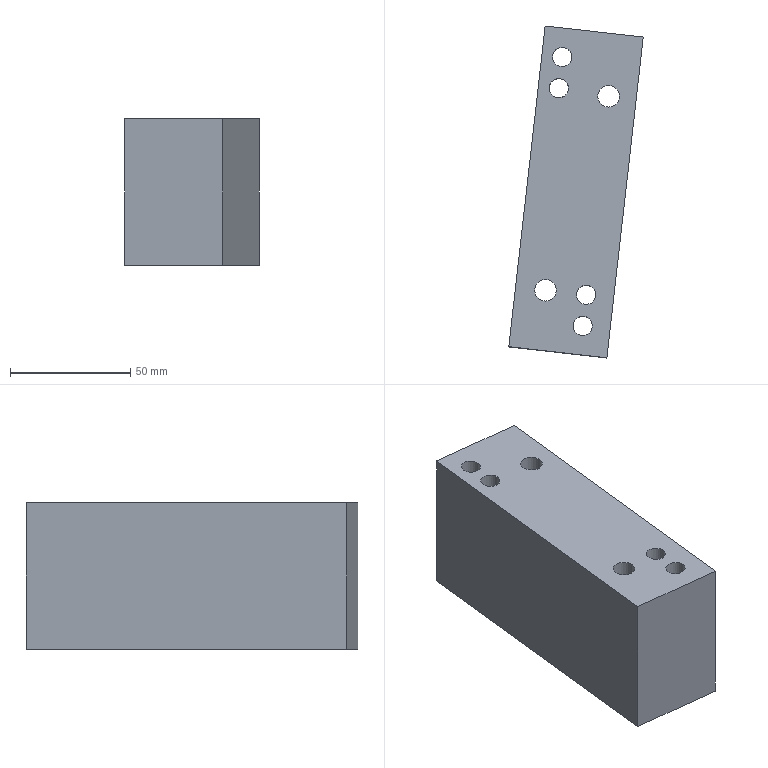Part | NX | features TB 2 | 1 solid | 20 faces | box 55.812 x 137.761 x 61 mm | volume 305856 mm3 | cylinder 10 | plane 8 | cone 2 | commonest cylinder face diameters 8.001 x4 6.8 x2 9 x2 14.5 x2
STEP:
#1=CARTESIAN_POINT('',(219.308,-204.553,40.));
#2=VERTEX_POINT('',#1);
#3=CARTESIAN_POINT('',(219.308,-208.553,40.));
#4=DIRECTION('',(0.,0.,-1.));
#5=DIRECTION('',(0.,1.,0.));
#6=AXIS2_PLACEMENT_3D('',#3,#4,#5);
#7=CIRCLE('',#6,4.);
#8=EDGE_CURVE('',#2,#2,#7,.T.);
#9=ORIENTED_EDGE('',*,*,#8,.F.);
#10=EDGE_LOOP('',(#9));
#11=FACE_BOUND('',#10,.T.);
#12=CARTESIAN_POINT('',(227.801,-316.217,40.));
#13=VERTEX_POINT('',#12);
#14=CARTESIAN_POINT('',(227.801,-320.217,40.));
#15=DIRECTION('',(0.,0.,-1.));
#16=DIRECTION('',(0.,1.,0.));
#17=AXIS2_PLACEMENT_3D('',#14,#15,#16);
#18=CIRCLE('',#17,4.);
#19=EDGE_CURVE('',#13,#13,#18,.T.);
#20=ORIENTED_EDGE('',*,*,#19,.F.);
#21=EDGE_LOOP('',(#20));
#22=FACE_BOUND('',#21,.T.);
#23=CARTESIAN_POINT('',(243.462,-211.909,40.));
#24=VERTEX_POINT('',#23);
#25=CARTESIAN_POINT('',(240.062,-211.909,40.));
#26=DIRECTION('',(0.,0.,1.));
#27=DIRECTION('',(1.,0.,0.));
#28=AXIS2_PLACEMENT_3D('',#25,#26,#27);
#29=CIRCLE('',#28,3.4);
#30=EDGE_CURVE('',#24,#24,#29,.T.);
#31=ORIENTED_EDGE('',*,*,#30,.T.);
#32=EDGE_LOOP('',(#31));
#33=FACE_BOUND('',#32,.T.);
#34=CARTESIAN_POINT('',(229.264,-303.299,40.));
#35=VERTEX_POINT('',#34);
#36=CARTESIAN_POINT('',(229.264,-307.3,40.));
#37=DIRECTION('',(0.,0.,1.));
#38=DIRECTION('',(0.,1.,0.));
#39=AXIS2_PLACEMENT_3D('',#36,#37,#38);
#40=CIRCLE('',#39,4.);
#41=EDGE_CURVE('',#35,#35,#40,.T.);
#42=ORIENTED_EDGE('',*,*,#41,.T.);
#43=EDGE_LOOP('',(#42));
#44=FACE_BOUND('',#43,.T.);
#45=CARTESIAN_POINT('',(212.371,-298.138,40.));
#46=VERTEX_POINT('',#45);
#47=CARTESIAN_POINT('',(212.371,-305.388,40.));
#48=DIRECTION('',(0.,0.,-1.));
#49=DIRECTION('',(0.,1.,0.));
#50=AXIS2_PLACEMENT_3D('',#47,#48,#49);
#51=CIRCLE('',#50,7.25);
#52=EDGE_CURVE('',#46,#46,#51,.T.);
#53=ORIENTED_EDGE('',*,*,#52,.F.);
#54=EDGE_LOOP('',(#53));
#55=FACE_BOUND('',#54,.T.);
#56=CARTESIAN_POINT('',(238.6,-217.577,40.));
#57=VERTEX_POINT('',#56);
#58=CARTESIAN_POINT('',(238.6,-224.827,40.));
#59=DIRECTION('',(0.,0.,1.));
#60=DIRECTION('',(0.,1.,0.));
#61=AXIS2_PLACEMENT_3D('',#58,#59,#60);
#62=CIRCLE('',#61,7.25);
#63=EDGE_CURVE('',#57,#57,#62,.T.);
#64=ORIENTED_EDGE('',*,*,#63,.T.);
#65=EDGE_LOOP('',(#64));
#66=FACE_BOUND('',#65,.T.);
#67=CARTESIAN_POINT('',(197.139,-328.823,40.));
#68=VERTEX_POINT('',#67);
#69=CARTESIAN_POINT('',(237.879,-333.435,40.));
#70=VERTEX_POINT('',#69);
#71=CARTESIAN_POINT('',(443.385,-356.698,40.));
#72=DIRECTION('',(0.9937,-0.1125,0.));
#73=VECTOR('',#72,1000.);
#74=LINE('',#71,#73);
#75=EDGE_CURVE('',#68,#70,#74,.T.);
#76=ORIENTED_EDGE('',*,*,#75,.F.);
#77=CARTESIAN_POINT('',(212.211,-195.673,40.));
#78=VERTEX_POINT('',#77);
#79=CARTESIAN_POINT('',(174.024,-533.017,40.));
#80=DIRECTION('',(-0.1125,-0.9937,0.));
#81=VECTOR('',#80,1000.);
#82=LINE('',#79,#81);
#83=EDGE_CURVE('',#78,#68,#82,.T.);
#84=ORIENTED_EDGE('',*,*,#83,.F.);
#85=CARTESIAN_POINT('',(252.951,-200.285,40.));
#86=VERTEX_POINT('',#85);
#87=CARTESIAN_POINT('',(458.458,-223.548,40.));
#88=DIRECTION('',(-0.9937,0.1125,0.));
#89=VECTOR('',#88,1000.);
#90=LINE('',#87,#89);
#91=EDGE_CURVE('',#86,#78,#90,.T.);
#92=ORIENTED_EDGE('',*,*,#91,.F.);
#93=CARTESIAN_POINT('',(214.764,-537.629,40.));
#94=DIRECTION('',(0.1125,0.9937,0.));
#95=VECTOR('',#94,1000.);
#96=LINE('',#93,#95);
#97=EDGE_CURVE('',#70,#86,#96,.T.);
#98=ORIENTED_EDGE('',*,*,#97,.F.);
#99=EDGE_LOOP('',(#76,#84,#92,#98));
#100=FACE_BOUND('',#99,.T.);
#101=CARTESIAN_POINT('',(217.845,-217.47,40.));
#102=VERTEX_POINT('',#101);
#103=CARTESIAN_POINT('',(217.845,-221.471,40.));
#104=DIRECTION('',(0.,0.,1.));
#105=DIRECTION('',(0.,1.,0.));
#106=AXIS2_PLACEMENT_3D('',#103,#104,#105);
#107=CIRCLE('',#106,4.);
#108=EDGE_CURVE('',#102,#102,#107,.T.);
#109=ORIENTED_EDGE('',*,*,#108,.T.);
#110=EDGE_LOOP('',(#109));
#111=FACE_BOUND('',#110,.T.);
#112=CARTESIAN_POINT('',(214.309,-318.305,40.));
#113=VERTEX_POINT('',#112);
#114=CARTESIAN_POINT('',(210.909,-318.305,40.));
#115=DIRECTION('',(0.,0.,1.));
#116=DIRECTION('',(1.,0.,0.));
#117=AXIS2_PLACEMENT_3D('',#114,#115,#116);
#118=CIRCLE('',#117,3.4);
#119=EDGE_CURVE('',#113,#113,#118,.T.);
#120=ORIENTED_EDGE('',*,*,#119,.T.);
#121=EDGE_LOOP('',(#120));
#122=FACE_BOUND('',#121,.T.);
#123=CARTESIAN_POINT('',(420.271,-560.892,40.));
#124=DIRECTION('',(0.,0.,-1.));
#125=DIRECTION('',(-0.9981,-0.06177,0.));
#126=AXIS2_PLACEMENT_3D('',#123,#124,#125);
#127=PLANE('',#126);
#128=ADVANCED_FACE('',(#11,#22,#33,#44,#55,#66,#100,#111,#122),#127,.T.);
#129=CARTESIAN_POINT('',(237.879,-333.435,101.));
#130=VERTEX_POINT('',#129);
#131=CARTESIAN_POINT('',(252.951,-200.285,101.));
#132=VERTEX_POINT('',#131);
#133=CARTESIAN_POINT('',(214.764,-537.629,101.));
#134=DIRECTION('',(0.1125,0.9937,0.));
#135=VECTOR('',#134,1000.);
#136=LINE('',#133,#135);
#137=EDGE_CURVE('',#130,#132,#136,.T.);
#138=ORIENTED_EDGE('',*,*,#137,.T.);
#139=CARTESIAN_POINT('',(212.211,-195.673,101.));
#140=VERTEX_POINT('',#139);
#141=CARTESIAN_POINT('',(458.458,-223.548,101.));
#142=DIRECTION('',(-0.9937,0.1125,0.));
#143=VECTOR('',#142,1000.);
#144=LINE('',#141,#143);
#145=EDGE_CURVE('',#132,#140,#144,.T.);
#146=ORIENTED_EDGE('',*,*,#145,.T.);
#147=CARTESIAN_POINT('',(197.139,-328.823,101.));
#148=VERTEX_POINT('',#147);
#149=CARTESIAN_POINT('',(174.024,-533.017,101.));
#150=DIRECTION('',(-0.1125,-0.9937,0.));
#151=VECTOR('',#150,1000.);
#152=LINE('',#149,#151);
#153=EDGE_CURVE('',#140,#148,#152,.T.);
#154=ORIENTED_EDGE('',*,*,#153,.T.);
#155=CARTESIAN_POINT('',(443.385,-356.698,101.));
#156=DIRECTION('',(0.9937,-0.1125,0.));
#157=VECTOR('',#156,1000.);
#158=LINE('',#155,#157);
#159=EDGE_CURVE('',#148,#130,#158,.T.);
#160=ORIENTED_EDGE('',*,*,#159,.T.);
#161=EDGE_LOOP('',(#138,#146,#154,#160));
#162=FACE_BOUND('',#161,.T.);
#163=CARTESIAN_POINT('',(238.6,-220.327,101.));
#164=VERTEX_POINT('',#163);
#165=CARTESIAN_POINT('',(238.6,-224.827,101.));
#166=DIRECTION('',(0.,0.,1.));
#167=DIRECTION('',(0.,1.,0.));
#168=AXIS2_PLACEMENT_3D('',#165,#166,#167);
#169=CIRCLE('',#168,4.5);
#170=EDGE_CURVE('',#164,#164,#169,.T.);
#171=ORIENTED_EDGE('',*,*,#170,.F.);
#172=EDGE_LOOP('',(#171));
#173=FACE_BOUND('',#172,.T.);
#174=CARTESIAN_POINT('',(212.371,-300.888,101.));
#175=VERTEX_POINT('',#174);
#176=CARTESIAN_POINT('',(212.371,-305.388,101.));
#177=DIRECTION('',(0.,0.,-1.));
#178=DIRECTION('',(0.,1.,0.));
#179=AXIS2_PLACEMENT_3D('',#176,#177,#178);
#180=CIRCLE('',#179,4.5);
#181=EDGE_CURVE('',#175,#175,#180,.T.);
#182=ORIENTED_EDGE('',*,*,#181,.T.);
#183=EDGE_LOOP('',(#182));
#184=FACE_BOUND('',#183,.T.);
#185=CARTESIAN_POINT('',(225.263,-307.3,101.));
#186=VERTEX_POINT('',#185);
#187=CARTESIAN_POINT('',(229.264,-307.3,101.));
#188=DIRECTION('',(0.,0.,-1.));
#189=DIRECTION('',(-1.,0.,0.));
#190=AXIS2_PLACEMENT_3D('',#187,#188,#189);
#191=CIRCLE('',#190,4.);
#192=EDGE_CURVE('',#186,#186,#191,.T.);
#193=ORIENTED_EDGE('',*,*,#192,.T.);
#194=EDGE_LOOP('',(#193));
#195=FACE_BOUND('',#194,.T.);
#196=CARTESIAN_POINT('',(221.846,-221.471,101.));
#197=VERTEX_POINT('',#196);
#198=CARTESIAN_POINT('',(217.845,-221.471,101.));
#199=DIRECTION('',(0.,0.,1.));
#200=DIRECTION('',(1.,0.,0.));
#201=AXIS2_PLACEMENT_3D('',#198,#199,#200);
#202=CIRCLE('',#201,4.);
#203=EDGE_CURVE('',#197,#197,#202,.T.);
#204=ORIENTED_EDGE('',*,*,#203,.F.);
#205=EDGE_LOOP('',(#204));
#206=FACE_BOUND('',#205,.T.);
#207=CARTESIAN_POINT('',(219.308,-204.553,101.));
#208=VERTEX_POINT('',#207);
#209=CARTESIAN_POINT('',(219.308,-208.553,101.));
#210=DIRECTION('',(0.,0.,1.));
#211=DIRECTION('',(0.,1.,0.));
#212=AXIS2_PLACEMENT_3D('',#209,#210,#211);
#213=CIRCLE('',#212,4.);
#214=EDGE_CURVE('',#208,#208,#213,.T.);
#215=ORIENTED_EDGE('',*,*,#214,.F.);
#216=EDGE_LOOP('',(#215));
#217=FACE_BOUND('',#216,.T.);
#218=CARTESIAN_POINT('',(227.801,-316.217,101.));
#219=VERTEX_POINT('',#218);
#220=CARTESIAN_POINT('',(227.801,-320.217,101.));
#221=DIRECTION('',(0.,0.,1.));
#222=DIRECTION('',(0.,1.,0.));
#223=AXIS2_PLACEMENT_3D('',#220,#221,#222);
#224=CIRCLE('',#223,4.);
#225=EDGE_CURVE('',#219,#219,#224,.T.);
#226=ORIENTED_EDGE('',*,*,#225,.F.);
#227=EDGE_LOOP('',(#226));
#228=FACE_BOUND('',#227,.T.);
#229=CARTESIAN_POINT('',(427.226,-561.68,101.));
#230=DIRECTION('',(0.,0.,-1.));
#231=DIRECTION('',(-0.9981,-0.06177,0.));
#232=AXIS2_PLACEMENT_3D('',#229,#230,#231);
#233=PLANE('',#232);
#234=ADVANCED_FACE('',(#162,#173,#184,#195,#206,#217,#228),#233,.F.);
#235=CARTESIAN_POINT('',(238.6,-217.577,81.));
#236=VERTEX_POINT('',#235);
#237=CARTESIAN_POINT('',(238.6,-224.827,81.));
#238=DIRECTION('',(0.,0.,-1.));
#239=DIRECTION('',(0.,1.,0.));
#240=AXIS2_PLACEMENT_3D('',#237,#238,#239);
#241=CIRCLE('',#240,7.25);
#242=EDGE_CURVE('',#236,#236,#241,.T.);
#243=ORIENTED_EDGE('',*,*,#242,.T.);
#244=EDGE_LOOP('',(#243));
#245=FACE_BOUND('',#244,.T.);
#246=CARTESIAN_POINT('',(238.6,-220.327,81.));
#247=VERTEX_POINT('',#246);
#248=CARTESIAN_POINT('',(238.6,-224.827,81.));
#249=DIRECTION('',(0.,0.,1.));
#250=DIRECTION('',(0.,1.,0.));
#251=AXIS2_PLACEMENT_3D('',#248,#249,#250);
#252=CIRCLE('',#251,4.5);
#253=EDGE_CURVE('',#247,#247,#252,.T.);
#254=ORIENTED_EDGE('',*,*,#253,.T.);
#255=EDGE_LOOP('',(#254));
#256=FACE_BOUND('',#255,.T.);
#257=CARTESIAN_POINT('',(222.27,-271.285,81.));
#258=DIRECTION('',(0.,0.,-1.));
#259=DIRECTION('',(0.9981,0.06177,0.));
#260=AXIS2_PLACEMENT_3D('',#257,#258,#259);
#261=PLANE('',#260);
#262=ADVANCED_FACE('',(#245,#256),#261,.T.);
#263=CARTESIAN_POINT('',(212.371,-300.888,81.));
#264=VERTEX_POINT('',#263);
#265=CARTESIAN_POINT('',(212.371,-305.388,81.));
#266=DIRECTION('',(0.,0.,-1.));
#267=DIRECTION('',(0.,1.,0.));
#268=AXIS2_PLACEMENT_3D('',#265,#266,#267);
#269=CIRCLE('',#268,4.5);
#270=EDGE_CURVE('',#264,#264,#269,.T.);
#271=ORIENTED_EDGE('',*,*,#270,.F.);
#272=EDGE_LOOP('',(#271));
#273=FACE_BOUND('',#272,.T.);
#274=CARTESIAN_POINT('',(212.371,-298.138,81.));
#275=VERTEX_POINT('',#274);
#276=CARTESIAN_POINT('',(212.371,-305.388,81.));
#277=DIRECTION('',(0.,0.,1.));
#278=DIRECTION('',(0.,1.,0.));
#279=AXIS2_PLACEMENT_3D('',#276,#277,#278);
#280=CIRCLE('',#279,7.25);
#281=EDGE_CURVE('',#275,#275,#280,.T.);
#282=ORIENTED_EDGE('',*,*,#281,.F.);
#283=EDGE_LOOP('',(#282));
#284=FACE_BOUND('',#283,.T.);
#285=CARTESIAN_POINT('',(222.27,-271.285,81.));
#286=DIRECTION('',(0.,0.,-1.));
#287=DIRECTION('',(0.9981,0.06177,0.));
#288=AXIS2_PLACEMENT_3D('',#285,#286,#287);
#289=PLANE('',#288);
#290=ADVANCED_FACE('',(#273,#284),#289,.T.);
#291=ORIENTED_EDGE('',*,*,#181,.F.);
#292=EDGE_LOOP('',(#291));
#293=FACE_BOUND('',#292,.T.);
#294=ORIENTED_EDGE('',*,*,#270,.T.);
#295=EDGE_LOOP('',(#294));
#296=FACE_BOUND('',#295,.T.);
#297=CARTESIAN_POINT('',(212.371,-305.388,86.));
#298=DIRECTION('',(0.,0.,1.));
#299=DIRECTION('',(-0.9981,-0.06177,0.));
#300=AXIS2_PLACEMENT_3D('',#297,#298,#299);
#301=CYLINDRICAL_SURFACE('',#300,4.5);
#302=ADVANCED_FACE('',(#293,#296),#301,.F.);
#303=ORIENTED_EDGE('',*,*,#170,.T.);
#304=EDGE_LOOP('',(#303));
#305=FACE_BOUND('',#304,.T.);
#306=ORIENTED_EDGE('',*,*,#253,.F.);
#307=EDGE_LOOP('',(#306));
#308=FACE_BOUND('',#307,.T.);
#309=CARTESIAN_POINT('',(238.6,-224.827,86.));
#310=DIRECTION('',(0.,0.,-1.));
#311=DIRECTION('',(0.9981,0.06177,0.));
#312=AXIS2_PLACEMENT_3D('',#309,#310,#311);
#313=CYLINDRICAL_SURFACE('',#312,4.5);
#314=ADVANCED_FACE('',(#305,#308),#313,.F.);
#315=ORIENTED_EDGE('',*,*,#153,.F.);
#316=CARTESIAN_POINT('',(212.211,-195.673,40.));
#317=DIRECTION('',(0.,0.,1.));
#318=VECTOR('',#317,1000.);
#319=LINE('',#316,#318);
#320=EDGE_CURVE('',#78,#140,#319,.T.);
#321=ORIENTED_EDGE('',*,*,#320,.F.);
#322=ORIENTED_EDGE('',*,*,#83,.T.);
#323=CARTESIAN_POINT('',(197.139,-328.823,40.));
#324=DIRECTION('',(0.,0.,1.));
#325=VECTOR('',#324,1000.);
#326=LINE('',#323,#325);
#327=EDGE_CURVE('',#68,#148,#326,.T.);
#328=ORIENTED_EDGE('',*,*,#327,.T.);
#329=EDGE_LOOP('',(#315,#321,#322,#328));
#330=FACE_BOUND('',#329,.T.);
#331=CARTESIAN_POINT('',(174.024,-533.017,40.));
#332=DIRECTION('',(-0.9937,0.1125,0.));
#333=DIRECTION('',(-0.1125,-0.9937,0.));
#334=AXIS2_PLACEMENT_3D('',#331,#332,#333);
#335=PLANE('',#334);
#336=ADVANCED_FACE('',(#330),#335,.T.);
#337=ORIENTED_EDGE('',*,*,#91,.T.);
#338=ORIENTED_EDGE('',*,*,#320,.T.);
#339=ORIENTED_EDGE('',*,*,#145,.F.);
#340=CARTESIAN_POINT('',(252.951,-200.285,40.));
#341=DIRECTION('',(0.,0.,1.));
#342=VECTOR('',#341,1000.);
#343=LINE('',#340,#342);
#344=EDGE_CURVE('',#86,#132,#343,.T.);
#345=ORIENTED_EDGE('',*,*,#344,.F.);
#346=EDGE_LOOP('',(#337,#338,#339,#345));
#347=FACE_BOUND('',#346,.T.);
#348=CARTESIAN_POINT('',(458.458,-223.548,40.));
#349=DIRECTION('',(0.1125,0.9937,0.));
#350=DIRECTION('',(-0.9937,0.1125,0.));
#351=AXIS2_PLACEMENT_3D('',#348,#349,#350);
#352=PLANE('',#351);
#353=ADVANCED_FACE('',(#347),#352,.T.);
#354=ORIENTED_EDGE('',*,*,#97,.T.);
#355=ORIENTED_EDGE('',*,*,#344,.T.);
#356=ORIENTED_EDGE('',*,*,#137,.F.);
#357=CARTESIAN_POINT('',(237.879,-333.435,40.));
#358=DIRECTION('',(0.,0.,1.));
#359=VECTOR('',#358,1000.);
#360=LINE('',#357,#359);
#361=EDGE_CURVE('',#70,#130,#360,.T.);
#362=ORIENTED_EDGE('',*,*,#361,.F.);
#363=EDGE_LOOP('',(#354,#355,#356,#362));
#364=FACE_BOUND('',#363,.T.);
#365=CARTESIAN_POINT('',(214.764,-537.629,40.));
#366=DIRECTION('',(0.9937,-0.1125,0.));
#367=DIRECTION('',(0.1125,0.9937,0.));
#368=AXIS2_PLACEMENT_3D('',#365,#366,#367);
#369=PLANE('',#368);
#370=ADVANCED_FACE('',(#364),#369,.T.);
#371=ORIENTED_EDGE('',*,*,#159,.F.);
#372=ORIENTED_EDGE('',*,*,#327,.F.);
#373=ORIENTED_EDGE('',*,*,#75,.T.);
#374=ORIENTED_EDGE('',*,*,#361,.T.);
#375=EDGE_LOOP('',(#371,#372,#373,#374));
#376=FACE_BOUND('',#375,.T.);
#377=CARTESIAN_POINT('',(443.385,-356.698,40.));
#378=DIRECTION('',(-0.1125,-0.9937,0.));
#379=DIRECTION('',(0.9937,-0.1125,0.));
#380=AXIS2_PLACEMENT_3D('',#377,#378,#379);
#381=PLANE('',#380);
#382=ADVANCED_FACE('',(#376),#381,.T.);
#383=ORIENTED_EDGE('',*,*,#242,.F.);
#384=EDGE_LOOP('',(#383));
#385=FACE_BOUND('',#384,.T.);
#386=ORIENTED_EDGE('',*,*,#63,.F.);
#387=EDGE_LOOP('',(#386));
#388=FACE_BOUND('',#387,.T.);
#389=CARTESIAN_POINT('',(238.6,-224.827,40.));
#390=DIRECTION('',(0.,0.,-1.));
#391=DIRECTION('',(0.9981,0.06177,0.));
#392=AXIS2_PLACEMENT_3D('',#389,#390,#391);
#393=CYLINDRICAL_SURFACE('',#392,7.25);
#394=ADVANCED_FACE('',(#385,#388),#393,.F.);
#395=ORIENTED_EDGE('',*,*,#281,.T.);
#396=EDGE_LOOP('',(#395));
#397=FACE_BOUND('',#396,.T.);
#398=ORIENTED_EDGE('',*,*,#52,.T.);
#399=EDGE_LOOP('',(#398));
#400=FACE_BOUND('',#399,.T.);
#401=CARTESIAN_POINT('',(212.371,-305.388,40.));
#402=DIRECTION('',(0.,0.,1.));
#403=DIRECTION('',(-0.9981,-0.06177,0.));
#404=AXIS2_PLACEMENT_3D('',#401,#402,#403);
#405=CYLINDRICAL_SURFACE('',#404,7.25);
#406=ADVANCED_FACE('',(#397,#400),#405,.F.);
#407=ORIENTED_EDGE('',*,*,#41,.F.);
#408=EDGE_LOOP('',(#407));
#409=FACE_BOUND('',#408,.T.);
#410=ORIENTED_EDGE('',*,*,#192,.F.);
#411=EDGE_LOOP('',(#410));
#412=FACE_BOUND('',#411,.T.);
#413=CARTESIAN_POINT('',(229.264,-307.3,30.));
#414=DIRECTION('',(0.,0.,1.));
#415=DIRECTION('',(0.,1.,0.));
#416=AXIS2_PLACEMENT_3D('',#413,#414,#415);
#417=CYLINDRICAL_SURFACE('',#416,4.);
#418=ADVANCED_FACE('',(#409,#412),#417,.F.);
#419=ORIENTED_EDGE('',*,*,#108,.F.);
#420=EDGE_LOOP('',(#419));
#421=FACE_BOUND('',#420,.T.);
#422=ORIENTED_EDGE('',*,*,#203,.T.);
#423=EDGE_LOOP('',(#422));
#424=FACE_BOUND('',#423,.T.);
#425=CARTESIAN_POINT('',(217.845,-221.471,30.));
#426=DIRECTION('',(0.,0.,1.));
#427=DIRECTION('',(0.,-1.,0.));
#428=AXIS2_PLACEMENT_3D('',#425,#426,#427);
#429=CYLINDRICAL_SURFACE('',#428,4.);
#430=ADVANCED_FACE('',(#421,#424),#429,.F.);
#431=CARTESIAN_POINT('',(240.062,-215.309,51.6));
#432=VERTEX_POINT('',#431);
#433=CARTESIAN_POINT('',(240.062,-211.909,51.6));
#434=DIRECTION('',(0.,0.,1.));
#435=DIRECTION('',(0.,-1.,0.));
#436=AXIS2_PLACEMENT_3D('',#433,#434,#435);
#437=CIRCLE('',#436,3.4);
#438=EDGE_CURVE('',#432,#432,#437,.T.);
#439=ORIENTED_EDGE('',*,*,#438,.T.);
#440=EDGE_LOOP('',(#439));
#441=FACE_BOUND('',#440,.T.);
#442=ORIENTED_EDGE('',*,*,#30,.F.);
#443=EDGE_LOOP('',(#442));
#444=FACE_BOUND('',#443,.T.);
#445=CARTESIAN_POINT('',(240.062,-211.909,40.));
#446=DIRECTION('',(0.,0.,1.));
#447=DIRECTION('',(-1.,0.,0.));
#448=AXIS2_PLACEMENT_3D('',#445,#446,#447);
#449=CYLINDRICAL_SURFACE('',#448,3.4);
#450=ADVANCED_FACE('',(#441,#444),#449,.F.);
#451=CARTESIAN_POINT('',(240.062,-211.909,55.));
#452=VERTEX_POINT('',#451);
#453=VERTEX_LOOP('',#452);
#454=FACE_BOUND('',#453,.T.);
#455=ORIENTED_EDGE('',*,*,#438,.F.);
#456=EDGE_LOOP('',(#455));
#457=FACE_BOUND('',#456,.T.);
#458=CARTESIAN_POINT('',(240.062,-211.909,51.6));
#459=DIRECTION('',(0.,0.,-1.));
#460=DIRECTION('',(0.,-1.,0.));
#461=AXIS2_PLACEMENT_3D('',#458,#459,#460);
#462=CONICAL_SURFACE('',#461,3.4,0.7854);
#463=ADVANCED_FACE('',(#454,#457),#462,.F.);
#464=CARTESIAN_POINT('',(210.909,-321.705,51.6));
#465=VERTEX_POINT('',#464);
#466=CARTESIAN_POINT('',(210.909,-318.305,51.6));
#467=DIRECTION('',(0.,0.,1.));
#468=DIRECTION('',(0.,-1.,0.));
#469=AXIS2_PLACEMENT_3D('',#466,#467,#468);
#470=CIRCLE('',#469,3.4);
#471=EDGE_CURVE('',#465,#465,#470,.T.);
#472=ORIENTED_EDGE('',*,*,#471,.T.);
#473=EDGE_LOOP('',(#472));
#474=FACE_BOUND('',#473,.T.);
#475=ORIENTED_EDGE('',*,*,#119,.F.);
#476=EDGE_LOOP('',(#475));
#477=FACE_BOUND('',#476,.T.);
#478=CARTESIAN_POINT('',(210.909,-318.305,40.));
#479=DIRECTION('',(0.,0.,1.));
#480=DIRECTION('',(-1.,0.,0.));
#481=AXIS2_PLACEMENT_3D('',#478,#479,#480);
#482=CYLINDRICAL_SURFACE('',#481,3.4);
#483=ADVANCED_FACE('',(#474,#477),#482,.F.);
#484=CARTESIAN_POINT('',(210.909,-318.305,55.));
#485=VERTEX_POINT('',#484);
#486=VERTEX_LOOP('',#485);
#487=FACE_BOUND('',#486,.T.);
#488=ORIENTED_EDGE('',*,*,#471,.F.);
#489=EDGE_LOOP('',(#488));
#490=FACE_BOUND('',#489,.T.);
#491=CARTESIAN_POINT('',(210.909,-318.305,51.6));
#492=DIRECTION('',(0.,0.,-1.));
#493=DIRECTION('',(0.,-1.,0.));
#494=AXIS2_PLACEMENT_3D('',#491,#492,#493);
#495=CONICAL_SURFACE('',#494,3.4,0.7854);
#496=ADVANCED_FACE('',(#487,#490),#495,.F.);
#497=ORIENTED_EDGE('',*,*,#19,.T.);
#498=EDGE_LOOP('',(#497));
#499=FACE_BOUND('',#498,.T.);
#500=ORIENTED_EDGE('',*,*,#225,.T.);
#501=EDGE_LOOP('',(#500));
#502=FACE_BOUND('',#501,.T.);
#503=CARTESIAN_POINT('',(227.801,-320.217,30.));
#504=DIRECTION('',(0.,0.,1.));
#505=DIRECTION('',(-1.,0.,0.));
#506=AXIS2_PLACEMENT_3D('',#503,#504,#505);
#507=CYLINDRICAL_SURFACE('',#506,4.);
#508=ADVANCED_FACE('',(#499,#502),#507,.F.);
#509=ORIENTED_EDGE('',*,*,#8,.T.);
#510=EDGE_LOOP('',(#509));
#511=FACE_BOUND('',#510,.T.);
#512=ORIENTED_EDGE('',*,*,#214,.T.);
#513=EDGE_LOOP('',(#512));
#514=FACE_BOUND('',#513,.T.);
#515=CARTESIAN_POINT('',(219.308,-208.553,30.));
#516=DIRECTION('',(0.,0.,1.));
#517=DIRECTION('',(-1.,0.,0.));
#518=AXIS2_PLACEMENT_3D('',#515,#516,#517);
#519=CYLINDRICAL_SURFACE('',#518,4.);
#520=ADVANCED_FACE('',(#511,#514),#519,.F.);
#521=CLOSED_SHELL('',(#128,#234,#262,#290,#302,#314,#336,#353,#370,#382,#394,#406,#418,#430,#450,#463,#483,#496,#508,#520));
#522=MANIFOLD_SOLID_BREP('',#521);
#523=(LENGTH_UNIT()NAMED_UNIT(*)SI_UNIT(.MILLI.,.METRE.));
#524=UNCERTAINTY_MEASURE_WITH_UNIT(LENGTH_MEASURE(0.00001),#523,'','');
#525=(NAMED_UNIT(*)PLANE_ANGLE_UNIT()SI_UNIT($,.RADIAN.));
#526=(NAMED_UNIT(*)SI_UNIT($,.STERADIAN.)SOLID_ANGLE_UNIT());
#527=(GEOMETRIC_REPRESENTATION_CONTEXT(3)GLOBAL_UNCERTAINTY_ASSIGNED_CONTEXT((#524))GLOBAL_UNIT_ASSIGNED_CONTEXT((#523,#525,#526))REPRESENTATION_CONTEXT('',''));
#528=ADVANCED_BREP_SHAPE_REPRESENTATION('',(#522),#527);